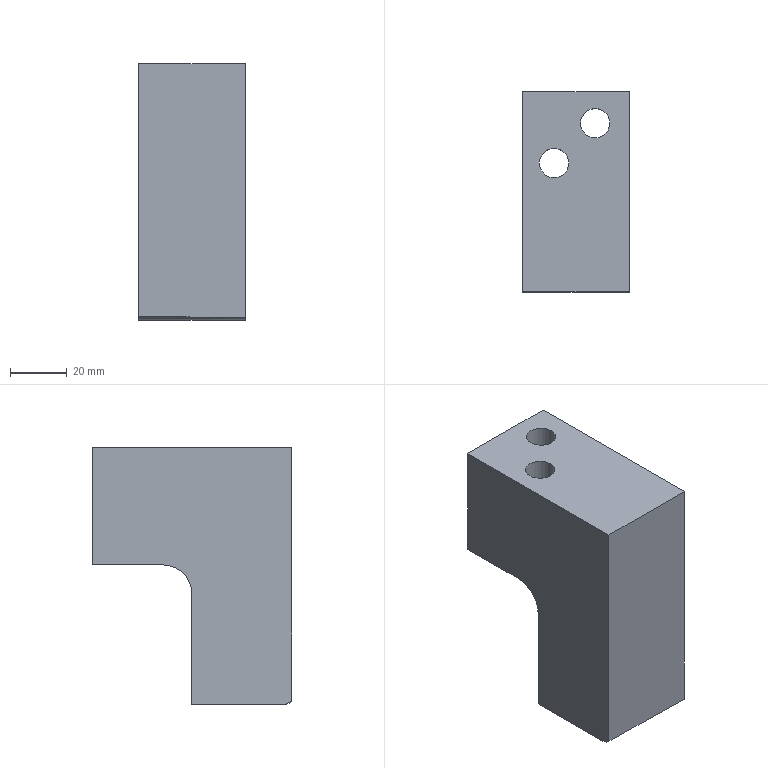Part | NX | features solid 2 | 1 solid | 16 faces | box 37.42 x 70.14 x 90.25 mm | volume 158061 mm3 | plane 10 | cylinder 6 | commonest cylinder face diameters 10.3 x2 17 x2 10 x1 20 x1
STEP:
#1=CARTESIAN_POINT('',(1200.146,183.154,48.));
#2=VERTEX_POINT('',#1);
#3=CARTESIAN_POINT('',(1194.996,183.154,48.));
#4=DIRECTION('',(0.,0.,1.));
#5=DIRECTION('',(1.,0.,0.));
#6=AXIS2_PLACEMENT_3D('',#3,#4,#5);
#7=CIRCLE('',#6,5.15);
#8=EDGE_CURVE('',#2,#2,#7,.F.);
#9=ORIENTED_EDGE('',*,*,#8,.T.);
#10=EDGE_LOOP('',(#9));
#11=FACE_BOUND('',#10,.T.);
#12=CARTESIAN_POINT('',(1200.146,183.154,60.));
#13=VERTEX_POINT('',#12);
#14=CARTESIAN_POINT('',(1194.996,183.154,60.));
#15=DIRECTION('',(0.,0.,1.));
#16=DIRECTION('',(1.,0.,0.));
#17=AXIS2_PLACEMENT_3D('',#14,#15,#16);
#18=CIRCLE('',#17,5.15);
#19=EDGE_CURVE('',#13,#13,#18,.F.);
#20=ORIENTED_EDGE('',*,*,#19,.F.);
#21=EDGE_LOOP('',(#20));
#22=FACE_BOUND('',#21,.T.);
#23=CARTESIAN_POINT('',(1194.996,183.154,53.75));
#24=DIRECTION('',(0.,0.,1.));
#25=DIRECTION('',(1.,0.,0.));
#26=AXIS2_PLACEMENT_3D('',#23,#24,#25);
#27=CYLINDRICAL_SURFACE('',#26,5.15);
#28=ADVANCED_FACE('',(#11,#22),#27,.F.);
#29=CARTESIAN_POINT('',(1185.726,169.154,48.));
#30=VERTEX_POINT('',#29);
#31=CARTESIAN_POINT('',(1180.576,169.154,48.));
#32=DIRECTION('',(0.,0.,1.));
#33=DIRECTION('',(1.,0.,0.));
#34=AXIS2_PLACEMENT_3D('',#31,#32,#33);
#35=CIRCLE('',#34,5.15);
#36=EDGE_CURVE('',#30,#30,#35,.F.);
#37=ORIENTED_EDGE('',*,*,#36,.T.);
#38=EDGE_LOOP('',(#37));
#39=FACE_BOUND('',#38,.T.);
#40=CARTESIAN_POINT('',(1185.726,169.154,60.));
#41=VERTEX_POINT('',#40);
#42=CARTESIAN_POINT('',(1180.576,169.154,60.));
#43=DIRECTION('',(0.,0.,1.));
#44=DIRECTION('',(1.,0.,0.));
#45=AXIS2_PLACEMENT_3D('',#42,#43,#44);
#46=CIRCLE('',#45,5.15);
#47=EDGE_CURVE('',#41,#41,#46,.F.);
#48=ORIENTED_EDGE('',*,*,#47,.F.);
#49=EDGE_LOOP('',(#48));
#50=FACE_BOUND('',#49,.T.);
#51=CARTESIAN_POINT('',(1180.576,169.154,53.75));
#52=DIRECTION('',(0.,0.,1.));
#53=DIRECTION('',(1.,0.,0.));
#54=AXIS2_PLACEMENT_3D('',#51,#52,#53);
#55=CYLINDRICAL_SURFACE('',#54,5.15);
#56=ADVANCED_FACE('',(#39,#50),#55,.F.);
#57=CARTESIAN_POINT('',(1206.996,124.014,-29.304));
#58=VERTEX_POINT('',#57);
#59=CARTESIAN_POINT('',(1206.996,124.014,60.));
#60=VERTEX_POINT('',#59);
#61=CARTESIAN_POINT('',(1206.996,124.014,-33.25));
#62=DIRECTION('',(0.,0.,1.));
#63=VECTOR('',#62,1000.);
#64=LINE('',#61,#63);
#65=EDGE_CURVE('',#58,#60,#64,.T.);
#66=ORIENTED_EDGE('',*,*,#65,.T.);
#67=CARTESIAN_POINT('',(1169.576,124.014,60.));
#68=VERTEX_POINT('',#67);
#69=CARTESIAN_POINT('',(1187.786,124.014,60.));
#70=DIRECTION('',(-1.,0.,0.));
#71=VECTOR('',#70,1000.);
#72=LINE('',#69,#71);
#73=EDGE_CURVE('',#60,#68,#72,.T.);
#74=ORIENTED_EDGE('',*,*,#73,.T.);
#75=CARTESIAN_POINT('',(1169.576,124.014,-28.741));
#76=VERTEX_POINT('',#75);
#77=CARTESIAN_POINT('',(1169.576,124.014,-33.25));
#78=DIRECTION('',(0.,0.,1.));
#79=VECTOR('',#78,1000.);
#80=LINE('',#77,#79);
#81=EDGE_CURVE('',#76,#68,#80,.T.);
#82=ORIENTED_EDGE('',*,*,#81,.F.);
#83=CARTESIAN_POINT('',(1374.691,124.014,-25.25));
#84=DIRECTION('',(0.,-1.,0.));
#85=DIRECTION('',(-1.,0.,0.));
#86=AXIS2_PLACEMENT_3D('',#83,#84,#85);
#87=ELLIPSE('',#86,286.493,5.);
#88=EDGE_CURVE('',#76,#58,#87,.T.);
#89=ORIENTED_EDGE('',*,*,#88,.T.);
#90=EDGE_LOOP('',(#66,#74,#82,#89));
#91=FACE_BOUND('',#90,.T.);
#92=CARTESIAN_POINT('',(1187.786,124.014,-33.25));
#93=DIRECTION('',(0.,-1.,0.));
#94=DIRECTION('',(0.,0.,1.));
#95=AXIS2_PLACEMENT_3D('',#92,#93,#94);
#96=PLANE('',#95);
#97=ADVANCED_FACE('',(#91),#96,.T.);
#98=CARTESIAN_POINT('',(1206.996,194.154,18.75));
#99=VERTEX_POINT('',#98);
#100=CARTESIAN_POINT('',(1206.996,194.154,60.));
#101=VERTEX_POINT('',#100);
#102=CARTESIAN_POINT('',(1206.996,194.154,-33.25));
#103=DIRECTION('',(0.,0.,1.));
#104=VECTOR('',#103,1000.);
#105=LINE('',#102,#104);
#106=EDGE_CURVE('',#99,#101,#105,.T.);
#107=ORIENTED_EDGE('',*,*,#106,.T.);
#108=CARTESIAN_POINT('',(1206.996,141.584,60.));
#109=DIRECTION('',(0.,-1.,0.));
#110=VECTOR('',#109,1000.);
#111=LINE('',#108,#110);
#112=EDGE_CURVE('',#101,#60,#111,.T.);
#113=ORIENTED_EDGE('',*,*,#112,.T.);
#114=ORIENTED_EDGE('',*,*,#65,.F.);
#115=CARTESIAN_POINT('',(1206.996,126.941,-30.25));
#116=VERTEX_POINT('',#115);
#117=CARTESIAN_POINT('',(1206.996,126.941,-25.25));
#118=DIRECTION('',(1.,0.,0.));
#119=DIRECTION('',(0.,1.,0.));
#120=AXIS2_PLACEMENT_3D('',#117,#118,#119);
#121=ELLIPSE('',#120,5.001,5.);
#122=EDGE_CURVE('',#58,#116,#121,.T.);
#123=ORIENTED_EDGE('',*,*,#122,.T.);
#124=CARTESIAN_POINT('',(1206.996,159.154,-30.25));
#125=VERTEX_POINT('',#124);
#126=CARTESIAN_POINT('',(1206.996,-1232.968,-30.25));
#127=DIRECTION('',(0.,1.,0.));
#128=VECTOR('',#127,1000.);
#129=LINE('',#126,#128);
#130=EDGE_CURVE('',#125,#116,#129,.F.);
#131=ORIENTED_EDGE('',*,*,#130,.F.);
#132=CARTESIAN_POINT('',(1206.996,159.154,8.75));
#133=VERTEX_POINT('',#132);
#134=CARTESIAN_POINT('',(1206.996,159.154,-33.25));
#135=DIRECTION('',(0.,0.,1.));
#136=VECTOR('',#135,1000.);
#137=LINE('',#134,#136);
#138=EDGE_CURVE('',#125,#133,#137,.T.);
#139=ORIENTED_EDGE('',*,*,#138,.T.);
#140=CARTESIAN_POINT('',(1206.996,169.154,18.75));
#141=VERTEX_POINT('',#140);
#142=CARTESIAN_POINT('',(1206.996,169.154,8.75));
#143=DIRECTION('',(1.,0.,0.));
#144=DIRECTION('',(0.,0.,-1.));
#145=AXIS2_PLACEMENT_3D('',#142,#143,#144);
#146=CIRCLE('',#145,10.);
#147=EDGE_CURVE('',#133,#141,#146,.F.);
#148=ORIENTED_EDGE('',*,*,#147,.T.);
#149=CARTESIAN_POINT('',(1206.996,141.584,18.75));
#150=DIRECTION('',(0.,1.,0.));
#151=VECTOR('',#150,1000.);
#152=LINE('',#149,#151);
#153=EDGE_CURVE('',#99,#141,#152,.F.);
#154=ORIENTED_EDGE('',*,*,#153,.F.);
#155=EDGE_LOOP('',(#107,#113,#114,#123,#131,#139,#148,#154));
#156=FACE_BOUND('',#155,.T.);
#157=CARTESIAN_POINT('',(1206.996,141.584,-33.25));
#158=DIRECTION('',(1.,0.,0.));
#159=DIRECTION('',(0.,0.,-1.));
#160=AXIS2_PLACEMENT_3D('',#157,#158,#159);
#161=PLANE('',#160);
#162=ADVANCED_FACE('',(#156),#161,.T.);
#163=CARTESIAN_POINT('',(1169.576,194.154,18.75));
#164=VERTEX_POINT('',#163);
#165=CARTESIAN_POINT('',(1169.576,194.154,60.));
#166=VERTEX_POINT('',#165);
#167=CARTESIAN_POINT('',(1169.576,194.154,-33.25));
#168=DIRECTION('',(0.,0.,1.));
#169=VECTOR('',#168,1000.);
#170=LINE('',#167,#169);
#171=EDGE_CURVE('',#164,#166,#170,.T.);
#172=ORIENTED_EDGE('',*,*,#171,.T.);
#173=CARTESIAN_POINT('',(1187.786,194.154,60.));
#174=DIRECTION('',(1.,0.,0.));
#175=VECTOR('',#174,1000.);
#176=LINE('',#173,#175);
#177=EDGE_CURVE('',#166,#101,#176,.T.);
#178=ORIENTED_EDGE('',*,*,#177,.T.);
#179=ORIENTED_EDGE('',*,*,#106,.F.);
#180=CARTESIAN_POINT('',(1187.786,194.154,18.75));
#181=DIRECTION('',(-1.,0.,0.));
#182=VECTOR('',#181,1000.);
#183=LINE('',#180,#182);
#184=EDGE_CURVE('',#164,#99,#183,.F.);
#185=ORIENTED_EDGE('',*,*,#184,.F.);
#186=EDGE_LOOP('',(#172,#178,#179,#185));
#187=FACE_BOUND('',#186,.T.);
#188=CARTESIAN_POINT('',(1187.786,194.154,-33.25));
#189=DIRECTION('',(0.,1.,0.));
#190=DIRECTION('',(0.,0.,-1.));
#191=AXIS2_PLACEMENT_3D('',#188,#189,#190);
#192=PLANE('',#191);
#193=ADVANCED_FACE('',(#187),#192,.T.);
#194=ORIENTED_EDGE('',*,*,#81,.T.);
#195=CARTESIAN_POINT('',(1169.576,141.584,60.));
#196=DIRECTION('',(0.,1.,0.));
#197=VECTOR('',#196,1000.);
#198=LINE('',#195,#197);
#199=EDGE_CURVE('',#68,#166,#198,.T.);
#200=ORIENTED_EDGE('',*,*,#199,.T.);
#201=ORIENTED_EDGE('',*,*,#171,.F.);
#202=CARTESIAN_POINT('',(1169.576,169.154,18.75));
#203=VERTEX_POINT('',#202);
#204=CARTESIAN_POINT('',(1169.576,159.154,18.75));
#205=DIRECTION('',(0.,1.,0.));
#206=VECTOR('',#205,1000.);
#207=LINE('',#204,#206);
#208=EDGE_CURVE('',#164,#203,#207,.F.);
#209=ORIENTED_EDGE('',*,*,#208,.T.);
#210=CARTESIAN_POINT('',(1169.576,159.154,8.75));
#211=VERTEX_POINT('',#210);
#212=CARTESIAN_POINT('',(1169.576,169.154,8.75));
#213=DIRECTION('',(-1.,0.,0.));
#214=DIRECTION('',(0.,0.,1.));
#215=AXIS2_PLACEMENT_3D('',#212,#213,#214);
#216=CIRCLE('',#215,10.);
#217=EDGE_CURVE('',#203,#211,#216,.F.);
#218=ORIENTED_EDGE('',*,*,#217,.T.);
#219=CARTESIAN_POINT('',(1169.576,159.154,-30.25));
#220=VERTEX_POINT('',#219);
#221=CARTESIAN_POINT('',(1169.576,159.154,-33.25));
#222=DIRECTION('',(0.,0.,1.));
#223=VECTOR('',#222,1000.);
#224=LINE('',#221,#223);
#225=EDGE_CURVE('',#220,#211,#224,.T.);
#226=ORIENTED_EDGE('',*,*,#225,.F.);
#227=CARTESIAN_POINT('',(1169.576,127.594,-30.25));
#228=VERTEX_POINT('',#227);
#229=CARTESIAN_POINT('',(1169.576,141.584,-30.25));
#230=DIRECTION('',(0.,-1.,0.));
#231=VECTOR('',#230,1000.);
#232=LINE('',#229,#231);
#233=EDGE_CURVE('',#228,#220,#232,.F.);
#234=ORIENTED_EDGE('',*,*,#233,.F.);
#235=CARTESIAN_POINT('',(1169.576,127.594,-25.25));
#236=DIRECTION('',(-1.,0.,0.));
#237=DIRECTION('',(0.,1.,0.));
#238=AXIS2_PLACEMENT_3D('',#235,#236,#237);
#239=ELLIPSE('',#238,5.001,5.);
#240=EDGE_CURVE('',#228,#76,#239,.T.);
#241=ORIENTED_EDGE('',*,*,#240,.T.);
#242=EDGE_LOOP('',(#194,#200,#201,#209,#218,#226,#234,#241));
#243=FACE_BOUND('',#242,.T.);
#244=CARTESIAN_POINT('',(1169.576,141.584,-33.25));
#245=DIRECTION('',(-1.,0.,0.));
#246=DIRECTION('',(0.,0.,1.));
#247=AXIS2_PLACEMENT_3D('',#244,#245,#246);
#248=PLANE('',#247);
#249=ADVANCED_FACE('',(#243),#248,.T.);
#250=ORIENTED_EDGE('',*,*,#8,.F.);
#251=EDGE_LOOP('',(#250));
#252=FACE_BOUND('',#251,.T.);
#253=CARTESIAN_POINT('',(1203.496,183.154,48.));
#254=VERTEX_POINT('',#253);
#255=CARTESIAN_POINT('',(1194.996,183.154,48.));
#256=DIRECTION('',(0.,0.,1.));
#257=DIRECTION('',(1.,0.,0.));
#258=AXIS2_PLACEMENT_3D('',#255,#256,#257);
#259=CIRCLE('',#258,8.5);
#260=EDGE_CURVE('',#254,#254,#259,.F.);
#261=ORIENTED_EDGE('',*,*,#260,.T.);
#262=EDGE_LOOP('',(#261));
#263=FACE_BOUND('',#262,.T.);
#264=CARTESIAN_POINT('',(1197.808,190.557,48.));
#265=DIRECTION('',(0.,0.,1.));
#266=DIRECTION('',(1.,0.,0.));
#267=AXIS2_PLACEMENT_3D('',#264,#265,#266);
#268=PLANE('',#267);
#269=ADVANCED_FACE('',(#252,#263),#268,.F.);
#270=CARTESIAN_POINT('',(1186.496,183.154,18.75));
#271=VERTEX_POINT('',#270);
#272=CARTESIAN_POINT('',(1203.496,183.154,18.75));
#273=VERTEX_POINT('',#272);
#274=CARTESIAN_POINT('',(1194.996,183.154,18.75));
#275=DIRECTION('',(0.,0.,-1.));
#276=DIRECTION('',(-1.,0.,0.));
#277=AXIS2_PLACEMENT_3D('',#274,#275,#276);
#278=CIRCLE('',#277,8.5);
#279=EDGE_CURVE('',#271,#273,#278,.F.);
#280=ORIENTED_EDGE('',*,*,#279,.F.);
#281=CARTESIAN_POINT('',(1194.996,183.154,18.75));
#282=DIRECTION('',(0.,0.,-1.));
#283=DIRECTION('',(-1.,0.,0.));
#284=AXIS2_PLACEMENT_3D('',#281,#282,#283);
#285=CIRCLE('',#284,8.5);
#286=EDGE_CURVE('',#273,#271,#285,.F.);
#287=ORIENTED_EDGE('',*,*,#286,.F.);
#288=EDGE_LOOP('',(#280,#287));
#289=FACE_BOUND('',#288,.T.);
#290=ORIENTED_EDGE('',*,*,#260,.F.);
#291=EDGE_LOOP('',(#290));
#292=FACE_BOUND('',#291,.T.);
#293=CARTESIAN_POINT('',(1194.996,183.154,18.75));
#294=DIRECTION('',(0.,0.,1.));
#295=DIRECTION('',(1.,0.,0.));
#296=AXIS2_PLACEMENT_3D('',#293,#294,#295);
#297=CYLINDRICAL_SURFACE('',#296,8.5);
#298=ADVANCED_FACE('',(#289,#292),#297,.F.);
#299=ORIENTED_EDGE('',*,*,#122,.F.);
#300=ORIENTED_EDGE('',*,*,#88,.F.);
#301=ORIENTED_EDGE('',*,*,#240,.F.);
#302=CARTESIAN_POINT('',(1187.773,127.276,-30.25));
#303=DIRECTION('',(-0.9998,0.01745,0.));
#304=VECTOR('',#303,1000.);
#305=LINE('',#302,#304);
#306=EDGE_CURVE('',#116,#228,#305,.T.);
#307=ORIENTED_EDGE('',*,*,#306,.F.);
#308=EDGE_LOOP('',(#299,#300,#301,#307));
#309=FACE_BOUND('',#308,.T.);
#310=CARTESIAN_POINT('',(1180.949,127.396,-25.25));
#311=DIRECTION('',(-0.9998,0.01745,0.));
#312=DIRECTION('',(-0.01745,-0.9998,0.));
#313=AXIS2_PLACEMENT_3D('',#310,#311,#312);
#314=CYLINDRICAL_SURFACE('',#313,5.);
#315=ADVANCED_FACE('',(#309),#314,.T.);
#316=ORIENTED_EDGE('',*,*,#130,.T.);
#317=ORIENTED_EDGE('',*,*,#306,.T.);
#318=ORIENTED_EDGE('',*,*,#233,.T.);
#319=CARTESIAN_POINT('',(1187.786,159.154,-30.25));
#320=DIRECTION('',(-1.,0.,0.));
#321=VECTOR('',#320,1000.);
#322=LINE('',#319,#321);
#323=EDGE_CURVE('',#220,#125,#322,.F.);
#324=ORIENTED_EDGE('',*,*,#323,.T.);
#325=EDGE_LOOP('',(#316,#317,#318,#324));
#326=FACE_BOUND('',#325,.T.);
#327=CARTESIAN_POINT('',(178.557,-1232.968,-30.25));
#328=DIRECTION('',(0.,0.,1.));
#329=DIRECTION('',(-0.2588,0.9659,0.));
#330=AXIS2_PLACEMENT_3D('',#327,#328,#329);
#331=PLANE('',#330);
#332=ADVANCED_FACE('',(#326),#331,.F.);
#333=ORIENTED_EDGE('',*,*,#225,.T.);
#334=CARTESIAN_POINT('',(1187.786,159.154,8.75));
#335=DIRECTION('',(-1.,0.,0.));
#336=VECTOR('',#335,1000.);
#337=LINE('',#334,#336);
#338=EDGE_CURVE('',#211,#133,#337,.F.);
#339=ORIENTED_EDGE('',*,*,#338,.T.);
#340=ORIENTED_EDGE('',*,*,#138,.F.);
#341=ORIENTED_EDGE('',*,*,#323,.F.);
#342=EDGE_LOOP('',(#333,#339,#340,#341));
#343=FACE_BOUND('',#342,.T.);
#344=CARTESIAN_POINT('',(1187.786,159.154,-33.25));
#345=DIRECTION('',(0.,1.,0.));
#346=DIRECTION('',(0.,0.,-1.));
#347=AXIS2_PLACEMENT_3D('',#344,#345,#346);
#348=PLANE('',#347);
#349=ADVANCED_FACE('',(#343),#348,.T.);
#350=CARTESIAN_POINT('',(1172.076,169.154,18.75));
#351=VERTEX_POINT('',#350);
#352=CARTESIAN_POINT('',(1187.786,169.154,18.75));
#353=DIRECTION('',(1.,0.,0.));
#354=VECTOR('',#353,1000.);
#355=LINE('',#352,#354);
#356=EDGE_CURVE('',#351,#203,#355,.F.);
#357=ORIENTED_EDGE('',*,*,#356,.F.);
#358=CARTESIAN_POINT('',(1189.076,169.154,18.75));
#359=VERTEX_POINT('',#358);
#360=CARTESIAN_POINT('',(1172.076,169.154,18.75));
#361=CARTESIAN_POINT('',(1172.076,167.947,18.75));
#362=CARTESIAN_POINT('',(1172.604,165.598,18.295));
#363=CARTESIAN_POINT('',(1174.525,162.917,16.734));
#364=CARTESIAN_POINT('',(1176.676,161.47,15.212));
#365=CARTESIAN_POINT('',(1178.778,160.786,14.238));
#366=CARTESIAN_POINT('',(1180.56,160.589,13.91));
#367=CARTESIAN_POINT('',(1182.353,160.782,14.231));
#368=CARTESIAN_POINT('',(1184.454,161.46,15.199));
#369=CARTESIAN_POINT('',(1186.616,162.907,16.726));
#370=CARTESIAN_POINT('',(1188.542,165.581,18.29));
#371=CARTESIAN_POINT('',(1189.076,167.947,18.75));
#372=CARTESIAN_POINT('',(1189.076,169.154,18.75));
#373=B_SPLINE_CURVE_WITH_KNOTS('',3,(#360,#361,#362,#363,#364,#365,#366,#367,#368,#369,#370,#371,#372),.UNSPECIFIED.,.F.,.F.,(4,1,1,1,1,1,1,1,1,1,4),(0.,0.00356,0.00712,0.01068,0.01246,0.01424,0.01602,0.0178,0.02136,0.02492,0.02848),.UNSPECIFIED.);
#374=EDGE_CURVE('',#351,#359,#373,.T.);
#375=ORIENTED_EDGE('',*,*,#374,.T.);
#376=CARTESIAN_POINT('',(1187.786,169.154,18.75));
#377=DIRECTION('',(1.,0.,0.));
#378=VECTOR('',#377,1000.);
#379=LINE('',#376,#378);
#380=EDGE_CURVE('',#141,#359,#379,.F.);
#381=ORIENTED_EDGE('',*,*,#380,.F.);
#382=ORIENTED_EDGE('',*,*,#147,.F.);
#383=ORIENTED_EDGE('',*,*,#338,.F.);
#384=ORIENTED_EDGE('',*,*,#217,.F.);
#385=EDGE_LOOP('',(#357,#375,#381,#382,#383,#384));
#386=FACE_BOUND('',#385,.T.);
#387=CARTESIAN_POINT('',(1187.786,169.154,8.75));
#388=DIRECTION('',(-1.,0.,0.));
#389=DIRECTION('',(0.,0.,1.));
#390=AXIS2_PLACEMENT_3D('',#387,#388,#389);
#391=CYLINDRICAL_SURFACE('',#390,10.);
#392=ADVANCED_FACE('',(#386),#391,.F.);
#393=ORIENTED_EDGE('',*,*,#380,.T.);
#394=CARTESIAN_POINT('',(1180.576,169.154,18.75));
#395=DIRECTION('',(0.,0.,-1.));
#396=DIRECTION('',(-1.,0.,0.));
#397=AXIS2_PLACEMENT_3D('',#394,#395,#396);
#398=CIRCLE('',#397,8.5);
#399=EDGE_CURVE('',#359,#351,#398,.F.);
#400=ORIENTED_EDGE('',*,*,#399,.T.);
#401=ORIENTED_EDGE('',*,*,#356,.T.);
#402=ORIENTED_EDGE('',*,*,#208,.F.);
#403=ORIENTED_EDGE('',*,*,#184,.T.);
#404=ORIENTED_EDGE('',*,*,#153,.T.);
#405=EDGE_LOOP('',(#393,#400,#401,#402,#403,#404));
#406=FACE_BOUND('',#405,.T.);
#407=ORIENTED_EDGE('',*,*,#286,.T.);
#408=ORIENTED_EDGE('',*,*,#279,.T.);
#409=EDGE_LOOP('',(#407,#408));
#410=FACE_BOUND('',#409,.T.);
#411=CARTESIAN_POINT('',(1187.786,159.154,18.75));
#412=DIRECTION('',(0.,0.,-1.));
#413=DIRECTION('',(-1.,0.,0.));
#414=AXIS2_PLACEMENT_3D('',#411,#412,#413);
#415=PLANE('',#414);
#416=ADVANCED_FACE('',(#406,#410),#415,.T.);
#417=CARTESIAN_POINT('',(1189.076,169.154,48.));
#418=VERTEX_POINT('',#417);
#419=CARTESIAN_POINT('',(1180.576,169.154,48.));
#420=DIRECTION('',(0.,0.,1.));
#421=DIRECTION('',(1.,0.,0.));
#422=AXIS2_PLACEMENT_3D('',#419,#420,#421);
#423=CIRCLE('',#422,8.5);
#424=EDGE_CURVE('',#418,#418,#423,.F.);
#425=ORIENTED_EDGE('',*,*,#424,.F.);
#426=EDGE_LOOP('',(#425));
#427=FACE_BOUND('',#426,.T.);
#428=ORIENTED_EDGE('',*,*,#399,.F.);
#429=ORIENTED_EDGE('',*,*,#374,.F.);
#430=EDGE_LOOP('',(#428,#429));
#431=FACE_BOUND('',#430,.T.);
#432=CARTESIAN_POINT('',(1180.576,169.154,18.75));
#433=DIRECTION('',(0.,0.,1.));
#434=DIRECTION('',(1.,0.,0.));
#435=AXIS2_PLACEMENT_3D('',#432,#433,#434);
#436=CYLINDRICAL_SURFACE('',#435,8.5);
#437=ADVANCED_FACE('',(#427,#431),#436,.F.);
#438=ORIENTED_EDGE('',*,*,#36,.F.);
#439=EDGE_LOOP('',(#438));
#440=FACE_BOUND('',#439,.T.);
#441=ORIENTED_EDGE('',*,*,#424,.T.);
#442=EDGE_LOOP('',(#441));
#443=FACE_BOUND('',#442,.T.);
#444=CARTESIAN_POINT('',(1182.808,175.557,48.));
#445=DIRECTION('',(0.,0.,1.));
#446=DIRECTION('',(1.,0.,0.));
#447=AXIS2_PLACEMENT_3D('',#444,#445,#446);
#448=PLANE('',#447);
#449=ADVANCED_FACE('',(#440,#443),#448,.F.);
#450=ORIENTED_EDGE('',*,*,#47,.T.);
#451=EDGE_LOOP('',(#450));
#452=FACE_BOUND('',#451,.T.);
#453=ORIENTED_EDGE('',*,*,#73,.F.);
#454=ORIENTED_EDGE('',*,*,#112,.F.);
#455=ORIENTED_EDGE('',*,*,#177,.F.);
#456=ORIENTED_EDGE('',*,*,#199,.F.);
#457=EDGE_LOOP('',(#453,#454,#455,#456));
#458=FACE_BOUND('',#457,.T.);
#459=ORIENTED_EDGE('',*,*,#19,.T.);
#460=EDGE_LOOP('',(#459));
#461=FACE_BOUND('',#460,.T.);
#462=CARTESIAN_POINT('',(1188.286,159.154,60.));
#463=DIRECTION('',(0.,0.,1.));
#464=DIRECTION('',(1.,0.,0.));
#465=AXIS2_PLACEMENT_3D('',#462,#463,#464);
#466=PLANE('',#465);
#467=ADVANCED_FACE('',(#452,#458,#461),#466,.T.);
#468=CLOSED_SHELL('',(#28,#56,#97,#162,#193,#249,#269,#298,#315,#332,#349,#392,#416,#437,#449,#467));
#469=MANIFOLD_SOLID_BREP('',#468);
#470=(LENGTH_UNIT()NAMED_UNIT(*)SI_UNIT(.MILLI.,.METRE.));
#471=UNCERTAINTY_MEASURE_WITH_UNIT(LENGTH_MEASURE(0.0508),#470,'','');
#472=(NAMED_UNIT(*)PLANE_ANGLE_UNIT()SI_UNIT($,.RADIAN.));
#473=(NAMED_UNIT(*)SI_UNIT($,.STERADIAN.)SOLID_ANGLE_UNIT());
#474=(GEOMETRIC_REPRESENTATION_CONTEXT(3)GLOBAL_UNCERTAINTY_ASSIGNED_CONTEXT((#471))GLOBAL_UNIT_ASSIGNED_CONTEXT((#470,#472,#473))REPRESENTATION_CONTEXT('',''));
#475=ADVANCED_BREP_SHAPE_REPRESENTATION('',(#469),#474);